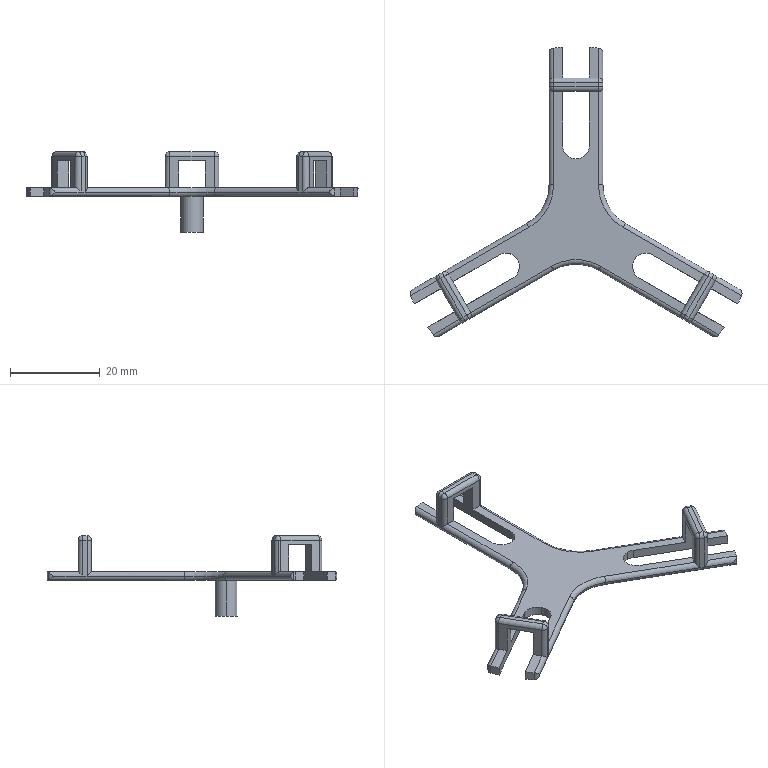Part | SolidWorks | features ICE 4, Fillet 3, CirPattern 1, Extrusion 1 | 1 solid | 117 faces | box 73.993 x 64.557 x 18 mm | volume 2470 mm3 | cylinder 66 | plane 33 | sphere 12 | torus 6 | commonest cylinder face diameters 2 x51 6 x7 80 x6 5 x2